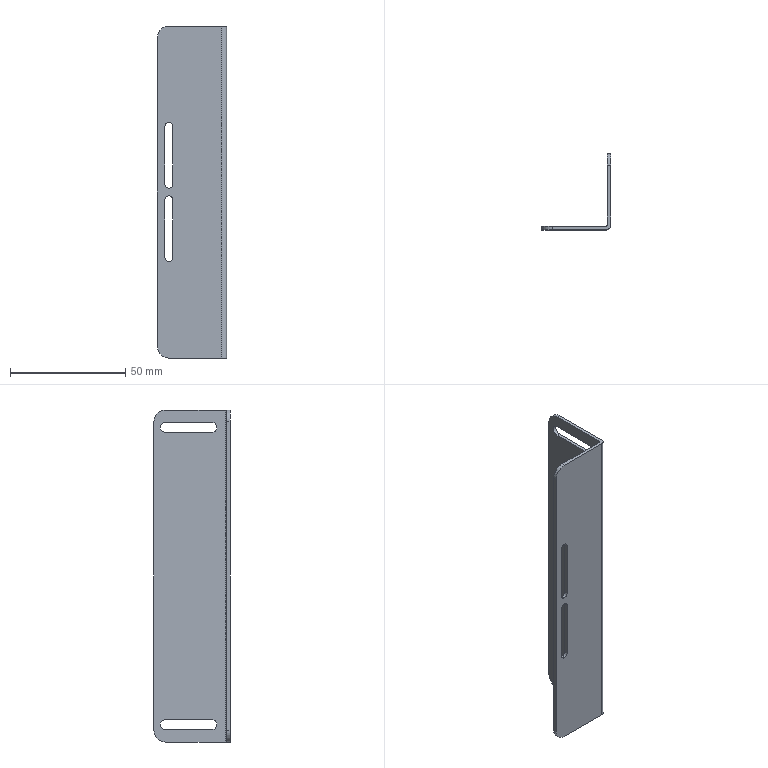Part | SolidWorks | features Fillet 3, ICE 2, Cut 1, Extrusion 1, Shell 1 | 1 solid | 32 faces | box 30 x 33 x 144 mm | volume 12527 mm3 | cylinder 16 | plane 16 | commonest cylinder face diameters 3.5 x6 4.5 x4 10 x4 1 x1 4 x1
STEP:
#1=CARTESIAN_POINT('',(6.75,1.5,43.625));
#2=VERTEX_POINT('',#1);
#3=CARTESIAN_POINT('',(5.,1.5,41.875));
#4=VERTEX_POINT('',#3);
#5=CARTESIAN_POINT('',(5.,1.5,43.625));
#6=DIRECTION('',(0.,1.,0.));
#7=DIRECTION('',(0.,0.,1.));
#8=AXIS2_PLACEMENT_3D('',#5,#6,#7);
#9=CIRCLE('',#8,1.75);
#10=EDGE_CURVE('',#2,#4,#9,.T.);
#11=ORIENTED_EDGE('',*,*,#10,.T.);
#12=CARTESIAN_POINT('',(5.,0.,41.875));
#13=VERTEX_POINT('',#12);
#14=CARTESIAN_POINT('',(5.,33.001,41.875));
#15=DIRECTION('',(0.,-1.,0.));
#16=VECTOR('',#15,1000.);
#17=LINE('',#14,#16);
#18=EDGE_CURVE('',#4,#13,#17,.T.);
#19=ORIENTED_EDGE('',*,*,#18,.T.);
#20=CARTESIAN_POINT('',(6.75,0.,43.625));
#21=VERTEX_POINT('',#20);
#22=CARTESIAN_POINT('',(5.,0.,43.625));
#23=DIRECTION('',(0.,1.,0.));
#24=DIRECTION('',(0.,0.,1.));
#25=AXIS2_PLACEMENT_3D('',#22,#23,#24);
#26=CIRCLE('',#25,1.75);
#27=EDGE_CURVE('',#21,#13,#26,.T.);
#28=ORIENTED_EDGE('',*,*,#27,.F.);
#29=CARTESIAN_POINT('',(6.75,33.001,43.625));
#30=DIRECTION('',(0.,-1.,0.));
#31=VECTOR('',#30,1000.);
#32=LINE('',#29,#31);
#33=EDGE_CURVE('',#2,#21,#32,.T.);
#34=ORIENTED_EDGE('',*,*,#33,.F.);
#35=EDGE_LOOP('',(#11,#19,#28,#34));
#36=FACE_OUTER_BOUND('',#35,.T.);
#37=CARTESIAN_POINT('',(5.,33.001,43.625));
#38=DIRECTION('',(0.,-1.,0.));
#39=DIRECTION('',(0.,0.,-1.));
#40=AXIS2_PLACEMENT_3D('',#37,#38,#39);
#41=CYLINDRICAL_SURFACE('',#40,1.75);
#42=ADVANCED_FACE('',(#36),#41,.F.);
#43=CARTESIAN_POINT('',(6.75,1.5,75.375));
#44=VERTEX_POINT('',#43);
#45=CARTESIAN_POINT('',(5.,1.5,73.625));
#46=VERTEX_POINT('',#45);
#47=CARTESIAN_POINT('',(5.,1.5,75.375));
#48=DIRECTION('',(0.,1.,0.));
#49=DIRECTION('',(0.,0.,1.));
#50=AXIS2_PLACEMENT_3D('',#47,#48,#49);
#51=CIRCLE('',#50,1.75);
#52=EDGE_CURVE('',#44,#46,#51,.T.);
#53=ORIENTED_EDGE('',*,*,#52,.T.);
#54=CARTESIAN_POINT('',(5.,0.,73.625));
#55=VERTEX_POINT('',#54);
#56=CARTESIAN_POINT('',(5.,33.001,73.625));
#57=DIRECTION('',(0.,-1.,0.));
#58=VECTOR('',#57,1000.);
#59=LINE('',#56,#58);
#60=EDGE_CURVE('',#46,#55,#59,.T.);
#61=ORIENTED_EDGE('',*,*,#60,.T.);
#62=CARTESIAN_POINT('',(6.75,0.,75.375));
#63=VERTEX_POINT('',#62);
#64=CARTESIAN_POINT('',(5.,0.,75.375));
#65=DIRECTION('',(0.,1.,0.));
#66=DIRECTION('',(0.,0.,1.));
#67=AXIS2_PLACEMENT_3D('',#64,#65,#66);
#68=CIRCLE('',#67,1.75);
#69=EDGE_CURVE('',#63,#55,#68,.T.);
#70=ORIENTED_EDGE('',*,*,#69,.F.);
#71=CARTESIAN_POINT('',(6.75,33.001,75.375));
#72=DIRECTION('',(0.,-1.,0.));
#73=VECTOR('',#72,1000.);
#74=LINE('',#71,#73);
#75=EDGE_CURVE('',#44,#63,#74,.T.);
#76=ORIENTED_EDGE('',*,*,#75,.F.);
#77=EDGE_LOOP('',(#53,#61,#70,#76));
#78=FACE_OUTER_BOUND('',#77,.T.);
#79=CARTESIAN_POINT('',(5.,33.001,75.375));
#80=DIRECTION('',(0.,-1.,0.));
#81=DIRECTION('',(0.,0.,-1.));
#82=AXIS2_PLACEMENT_3D('',#79,#80,#81);
#83=CYLINDRICAL_SURFACE('',#82,1.75);
#84=ADVANCED_FACE('',(#78),#83,.F.);
#85=ORIENTED_EDGE('',*,*,#69,.T.);
#86=CARTESIAN_POINT('',(3.25,0.,75.375));
#87=VERTEX_POINT('',#86);
#88=CARTESIAN_POINT('',(5.,0.,75.375));
#89=DIRECTION('',(0.,1.,0.));
#90=DIRECTION('',(0.,0.,1.));
#91=AXIS2_PLACEMENT_3D('',#88,#89,#90);
#92=CIRCLE('',#91,1.75);
#93=EDGE_CURVE('',#55,#87,#92,.T.);
#94=ORIENTED_EDGE('',*,*,#93,.T.);
#95=CARTESIAN_POINT('',(3.25,0.,100.375));
#96=VERTEX_POINT('',#95);
#97=CARTESIAN_POINT('',(3.25,0.,100.375));
#98=DIRECTION('',(0.,0.,1.));
#99=VECTOR('',#98,1000.);
#100=LINE('',#97,#99);
#101=EDGE_CURVE('',#87,#96,#100,.T.);
#102=ORIENTED_EDGE('',*,*,#101,.T.);
#103=CARTESIAN_POINT('',(6.75,0.,100.375));
#104=VERTEX_POINT('',#103);
#105=CARTESIAN_POINT('',(5.,0.,100.375));
#106=DIRECTION('',(0.,1.,0.));
#107=DIRECTION('',(0.,0.,1.));
#108=AXIS2_PLACEMENT_3D('',#105,#106,#107);
#109=CIRCLE('',#108,1.75);
#110=EDGE_CURVE('',#96,#104,#109,.T.);
#111=ORIENTED_EDGE('',*,*,#110,.T.);
#112=CARTESIAN_POINT('',(6.75,0.,100.375));
#113=DIRECTION('',(0.,0.,-1.));
#114=VECTOR('',#113,1000.);
#115=LINE('',#112,#114);
#116=EDGE_CURVE('',#104,#63,#115,.T.);
#117=ORIENTED_EDGE('',*,*,#116,.T.);
#118=EDGE_LOOP('',(#85,#94,#102,#111,#117));
#119=FACE_BOUND('',#118,.T.);
#120=CARTESIAN_POINT('',(5.,0.,0.));
#121=VERTEX_POINT('',#120);
#122=CARTESIAN_POINT('',(28.,0.,0.));
#123=VERTEX_POINT('',#122);
#124=CARTESIAN_POINT('',(0.,0.,0.));
#125=DIRECTION('',(1.,0.,0.));
#126=VECTOR('',#125,1000.);
#127=LINE('',#124,#126);
#128=EDGE_CURVE('',#121,#123,#127,.T.);
#129=ORIENTED_EDGE('',*,*,#128,.T.);
#130=CARTESIAN_POINT('',(28.,0.,144.));
#131=VERTEX_POINT('',#130);
#132=CARTESIAN_POINT('',(28.,0.,144.));
#133=DIRECTION('',(0.,0.,1.));
#134=VECTOR('',#133,1000.);
#135=LINE('',#132,#134);
#136=EDGE_CURVE('',#123,#131,#135,.T.);
#137=ORIENTED_EDGE('',*,*,#136,.T.);
#138=CARTESIAN_POINT('',(5.,0.,144.));
#139=VERTEX_POINT('',#138);
#140=CARTESIAN_POINT('',(0.,0.,144.));
#141=DIRECTION('',(1.,0.,0.));
#142=VECTOR('',#141,1000.);
#143=LINE('',#140,#142);
#144=EDGE_CURVE('',#139,#131,#143,.T.);
#145=ORIENTED_EDGE('',*,*,#144,.F.);
#146=CARTESIAN_POINT('',(0.,0.,139.));
#147=VERTEX_POINT('',#146);
#148=CARTESIAN_POINT('',(5.,0.,139.));
#149=DIRECTION('',(0.,-1.,0.));
#150=DIRECTION('',(0.,0.,1.));
#151=AXIS2_PLACEMENT_3D('',#148,#149,#150);
#152=CIRCLE('',#151,5.);
#153=EDGE_CURVE('',#139,#147,#152,.T.);
#154=ORIENTED_EDGE('',*,*,#153,.T.);
#155=CARTESIAN_POINT('',(0.,0.,5.));
#156=VERTEX_POINT('',#155);
#157=CARTESIAN_POINT('',(0.,0.,144.));
#158=DIRECTION('',(0.,0.,-1.));
#159=VECTOR('',#158,1000.);
#160=LINE('',#157,#159);
#161=EDGE_CURVE('',#147,#156,#160,.T.);
#162=ORIENTED_EDGE('',*,*,#161,.T.);
#163=CARTESIAN_POINT('',(5.,0.,5.));
#164=DIRECTION('',(0.,-1.,0.));
#165=DIRECTION('',(0.,0.,1.));
#166=AXIS2_PLACEMENT_3D('',#163,#164,#165);
#167=CIRCLE('',#166,5.);
#168=EDGE_CURVE('',#156,#121,#167,.T.);
#169=ORIENTED_EDGE('',*,*,#168,.T.);
#170=EDGE_LOOP('',(#129,#137,#145,#154,#162,#169));
#171=FACE_OUTER_BOUND('',#170,.T.);
#172=ORIENTED_EDGE('',*,*,#27,.T.);
#173=CARTESIAN_POINT('',(3.25,0.,43.625));
#174=VERTEX_POINT('',#173);
#175=CARTESIAN_POINT('',(5.,0.,43.625));
#176=DIRECTION('',(0.,1.,0.));
#177=DIRECTION('',(0.,0.,1.));
#178=AXIS2_PLACEMENT_3D('',#175,#176,#177);
#179=CIRCLE('',#178,1.75);
#180=EDGE_CURVE('',#13,#174,#179,.T.);
#181=ORIENTED_EDGE('',*,*,#180,.T.);
#182=CARTESIAN_POINT('',(3.25,0.,68.625));
#183=VERTEX_POINT('',#182);
#184=CARTESIAN_POINT('',(3.25,0.,68.625));
#185=DIRECTION('',(0.,0.,1.));
#186=VECTOR('',#185,1000.);
#187=LINE('',#184,#186);
#188=EDGE_CURVE('',#174,#183,#187,.T.);
#189=ORIENTED_EDGE('',*,*,#188,.T.);
#190=CARTESIAN_POINT('',(6.75,0.,68.625));
#191=VERTEX_POINT('',#190);
#192=CARTESIAN_POINT('',(5.,0.,68.625));
#193=DIRECTION('',(0.,1.,0.));
#194=DIRECTION('',(0.,0.,1.));
#195=AXIS2_PLACEMENT_3D('',#192,#193,#194);
#196=CIRCLE('',#195,1.75);
#197=EDGE_CURVE('',#183,#191,#196,.T.);
#198=ORIENTED_EDGE('',*,*,#197,.T.);
#199=CARTESIAN_POINT('',(6.75,0.,68.625));
#200=DIRECTION('',(0.,0.,-1.));
#201=VECTOR('',#200,1000.);
#202=LINE('',#199,#201);
#203=EDGE_CURVE('',#191,#21,#202,.T.);
#204=ORIENTED_EDGE('',*,*,#203,.T.);
#205=EDGE_LOOP('',(#172,#181,#189,#198,#204));
#206=FACE_BOUND('',#205,.T.);
#207=CARTESIAN_POINT('',(0.,0.,144.));
#208=DIRECTION('',(0.,1.,0.));
#209=DIRECTION('',(0.,0.,1.));
#210=AXIS2_PLACEMENT_3D('',#207,#208,#209);
#211=PLANE('',#210);
#212=ADVANCED_FACE('',(#119,#171,#206),#211,.F.);
#213=CARTESIAN_POINT('',(3.25,1.5,75.375));
#214=VERTEX_POINT('',#213);
#215=CARTESIAN_POINT('',(3.25,1.5,100.375));
#216=VERTEX_POINT('',#215);
#217=CARTESIAN_POINT('',(3.25,1.5,100.375));
#218=DIRECTION('',(0.,0.,1.));
#219=VECTOR('',#218,1000.);
#220=LINE('',#217,#219);
#221=EDGE_CURVE('',#214,#216,#220,.T.);
#222=ORIENTED_EDGE('',*,*,#221,.F.);
#223=CARTESIAN_POINT('',(5.,1.5,75.375));
#224=DIRECTION('',(0.,1.,0.));
#225=DIRECTION('',(0.,0.,1.));
#226=AXIS2_PLACEMENT_3D('',#223,#224,#225);
#227=CIRCLE('',#226,1.75);
#228=EDGE_CURVE('',#46,#214,#227,.T.);
#229=ORIENTED_EDGE('',*,*,#228,.F.);
#230=ORIENTED_EDGE('',*,*,#52,.F.);
#231=CARTESIAN_POINT('',(6.75,1.5,100.375));
#232=VERTEX_POINT('',#231);
#233=CARTESIAN_POINT('',(6.75,1.5,100.375));
#234=DIRECTION('',(0.,0.,-1.));
#235=VECTOR('',#234,1000.);
#236=LINE('',#233,#235);
#237=EDGE_CURVE('',#232,#44,#236,.T.);
#238=ORIENTED_EDGE('',*,*,#237,.F.);
#239=CARTESIAN_POINT('',(5.,1.5,100.375));
#240=DIRECTION('',(0.,1.,0.));
#241=DIRECTION('',(0.,0.,1.));
#242=AXIS2_PLACEMENT_3D('',#239,#240,#241);
#243=CIRCLE('',#242,1.75);
#244=EDGE_CURVE('',#216,#232,#243,.T.);
#245=ORIENTED_EDGE('',*,*,#244,.F.);
#246=EDGE_LOOP('',(#222,#229,#230,#238,#245));
#247=FACE_BOUND('',#246,.T.);
#248=CARTESIAN_POINT('',(5.,1.5,144.));
#249=VERTEX_POINT('',#248);
#250=CARTESIAN_POINT('',(28.,1.5,144.));
#251=VERTEX_POINT('',#250);
#252=CARTESIAN_POINT('',(0.,1.5,144.));
#253=DIRECTION('',(1.,0.,0.));
#254=VECTOR('',#253,1000.);
#255=LINE('',#252,#254);
#256=EDGE_CURVE('',#249,#251,#255,.T.);
#257=ORIENTED_EDGE('',*,*,#256,.T.);
#258=CARTESIAN_POINT('',(28.,1.5,0.));
#259=VERTEX_POINT('',#258);
#260=CARTESIAN_POINT('',(28.,1.5,0.));
#261=DIRECTION('',(0.,0.,-1.));
#262=VECTOR('',#261,1000.);
#263=LINE('',#260,#262);
#264=EDGE_CURVE('',#251,#259,#263,.T.);
#265=ORIENTED_EDGE('',*,*,#264,.T.);
#266=CARTESIAN_POINT('',(5.,1.5,0.));
#267=VERTEX_POINT('',#266);
#268=CARTESIAN_POINT('',(0.,1.5,0.));
#269=DIRECTION('',(1.,0.,0.));
#270=VECTOR('',#269,1000.);
#271=LINE('',#268,#270);
#272=EDGE_CURVE('',#267,#259,#271,.T.);
#273=ORIENTED_EDGE('',*,*,#272,.F.);
#274=CARTESIAN_POINT('',(0.,1.5,5.));
#275=VERTEX_POINT('',#274);
#276=CARTESIAN_POINT('',(5.,1.5,5.));
#277=DIRECTION('',(0.,1.,0.));
#278=DIRECTION('',(0.,0.,1.));
#279=AXIS2_PLACEMENT_3D('',#276,#277,#278);
#280=CIRCLE('',#279,5.);
#281=EDGE_CURVE('',#267,#275,#280,.T.);
#282=ORIENTED_EDGE('',*,*,#281,.T.);
#283=CARTESIAN_POINT('',(0.,1.5,139.));
#284=VERTEX_POINT('',#283);
#285=CARTESIAN_POINT('',(0.,1.5,144.));
#286=DIRECTION('',(0.,0.,-1.));
#287=VECTOR('',#286,1000.);
#288=LINE('',#285,#287);
#289=EDGE_CURVE('',#284,#275,#288,.T.);
#290=ORIENTED_EDGE('',*,*,#289,.F.);
#291=CARTESIAN_POINT('',(5.,1.5,139.));
#292=DIRECTION('',(0.,1.,0.));
#293=DIRECTION('',(0.,0.,1.));
#294=AXIS2_PLACEMENT_3D('',#291,#292,#293);
#295=CIRCLE('',#294,5.);
#296=EDGE_CURVE('',#284,#249,#295,.T.);
#297=ORIENTED_EDGE('',*,*,#296,.T.);
#298=EDGE_LOOP('',(#257,#265,#273,#282,#290,#297));
#299=FACE_OUTER_BOUND('',#298,.T.);
#300=CARTESIAN_POINT('',(3.25,1.5,43.625));
#301=VERTEX_POINT('',#300);
#302=CARTESIAN_POINT('',(3.25,1.5,68.625));
#303=VERTEX_POINT('',#302);
#304=CARTESIAN_POINT('',(3.25,1.5,68.625));
#305=DIRECTION('',(0.,0.,1.));
#306=VECTOR('',#305,1000.);
#307=LINE('',#304,#306);
#308=EDGE_CURVE('',#301,#303,#307,.T.);
#309=ORIENTED_EDGE('',*,*,#308,.F.);
#310=CARTESIAN_POINT('',(5.,1.5,43.625));
#311=DIRECTION('',(0.,1.,0.));
#312=DIRECTION('',(0.,0.,1.));
#313=AXIS2_PLACEMENT_3D('',#310,#311,#312);
#314=CIRCLE('',#313,1.75);
#315=EDGE_CURVE('',#4,#301,#314,.T.);
#316=ORIENTED_EDGE('',*,*,#315,.F.);
#317=ORIENTED_EDGE('',*,*,#10,.F.);
#318=CARTESIAN_POINT('',(6.75,1.5,68.625));
#319=VERTEX_POINT('',#318);
#320=CARTESIAN_POINT('',(6.75,1.5,68.625));
#321=DIRECTION('',(0.,0.,-1.));
#322=VECTOR('',#321,1000.);
#323=LINE('',#320,#322);
#324=EDGE_CURVE('',#319,#2,#323,.T.);
#325=ORIENTED_EDGE('',*,*,#324,.F.);
#326=CARTESIAN_POINT('',(5.,1.5,68.625));
#327=DIRECTION('',(0.,1.,0.));
#328=DIRECTION('',(0.,0.,1.));
#329=AXIS2_PLACEMENT_3D('',#326,#327,#328);
#330=CIRCLE('',#329,1.75);
#331=EDGE_CURVE('',#303,#319,#330,.T.);
#332=ORIENTED_EDGE('',*,*,#331,.F.);
#333=EDGE_LOOP('',(#309,#316,#317,#325,#332));
#334=FACE_BOUND('',#333,.T.);
#335=CARTESIAN_POINT('',(0.,1.5,144.));
#336=DIRECTION('',(0.,1.,0.));
#337=DIRECTION('',(0.,0.,1.));
#338=AXIS2_PLACEMENT_3D('',#335,#336,#337);
#339=PLANE('',#338);
#340=ADVANCED_FACE('',(#247,#299,#334),#339,.T.);
#341=CARTESIAN_POINT('',(28.5,33.,139.));
#342=VERTEX_POINT('',#341);
#343=CARTESIAN_POINT('',(28.5,33.,5.));
#344=VERTEX_POINT('',#343);
#345=CARTESIAN_POINT('',(28.5,33.,144.));
#346=DIRECTION('',(0.,0.,-1.));
#347=VECTOR('',#346,1000.);
#348=LINE('',#345,#347);
#349=EDGE_CURVE('',#342,#344,#348,.T.);
#350=ORIENTED_EDGE('',*,*,#349,.F.);
#351=CARTESIAN_POINT('',(30.,33.,139.));
#352=VERTEX_POINT('',#351);
#353=CARTESIAN_POINT('',(0.,33.,139.));
#354=DIRECTION('',(1.,0.,0.));
#355=VECTOR('',#354,1000.);
#356=LINE('',#353,#355);
#357=EDGE_CURVE('',#342,#352,#356,.T.);
#358=ORIENTED_EDGE('',*,*,#357,.T.);
#359=CARTESIAN_POINT('',(30.,33.,5.));
#360=VERTEX_POINT('',#359);
#361=CARTESIAN_POINT('',(30.,33.,144.));
#362=DIRECTION('',(0.,0.,-1.));
#363=VECTOR('',#362,1000.);
#364=LINE('',#361,#363);
#365=EDGE_CURVE('',#352,#360,#364,.T.);
#366=ORIENTED_EDGE('',*,*,#365,.T.);
#367=CARTESIAN_POINT('',(28.5,33.,5.));
#368=DIRECTION('',(-1.,0.,0.));
#369=VECTOR('',#368,1000.);
#370=LINE('',#367,#369);
#371=EDGE_CURVE('',#360,#344,#370,.T.);
#372=ORIENTED_EDGE('',*,*,#371,.T.);
#373=EDGE_LOOP('',(#350,#358,#366,#372));
#374=FACE_OUTER_BOUND('',#373,.T.);
#375=CARTESIAN_POINT('',(0.,33.,144.));
#376=DIRECTION('',(0.,-1.,0.));
#377=DIRECTION('',(0.,0.,-1.));
#378=AXIS2_PLACEMENT_3D('',#375,#376,#377);
#379=PLANE('',#378);
#380=ADVANCED_FACE('',(#374),#379,.F.);
#381=ORIENTED_EDGE('',*,*,#144,.T.);
#382=CARTESIAN_POINT('',(30.,2.,144.));
#383=VERTEX_POINT('',#382);
#384=CARTESIAN_POINT('',(28.,2.,144.));
#385=DIRECTION('',(0.,0.,1.));
#386=DIRECTION('',(-1.,0.,0.));
#387=AXIS2_PLACEMENT_3D('',#384,#385,#386);
#388=CIRCLE('',#387,2.);
#389=EDGE_CURVE('',#131,#383,#388,.T.);
#390=ORIENTED_EDGE('',*,*,#389,.T.);
#391=CARTESIAN_POINT('',(30.,28.,144.));
#392=VERTEX_POINT('',#391);
#393=CARTESIAN_POINT('',(30.,33.,144.));
#394=DIRECTION('',(0.,1.,0.));
#395=VECTOR('',#394,1000.);
#396=LINE('',#393,#395);
#397=EDGE_CURVE('',#383,#392,#396,.T.);
#398=ORIENTED_EDGE('',*,*,#397,.T.);
#399=CARTESIAN_POINT('',(28.5,28.,144.));
#400=VERTEX_POINT('',#399);
#401=CARTESIAN_POINT('',(0.,28.,144.));
#402=DIRECTION('',(-1.,0.,0.));
#403=VECTOR('',#402,1000.);
#404=LINE('',#401,#403);
#405=EDGE_CURVE('',#392,#400,#404,.T.);
#406=ORIENTED_EDGE('',*,*,#405,.T.);
#407=CARTESIAN_POINT('',(28.5,2.,144.));
#408=VERTEX_POINT('',#407);
#409=CARTESIAN_POINT('',(28.5,0.,144.));
#410=DIRECTION('',(0.,1.,0.));
#411=VECTOR('',#410,1000.);
#412=LINE('',#409,#411);
#413=EDGE_CURVE('',#408,#400,#412,.T.);
#414=ORIENTED_EDGE('',*,*,#413,.F.);
#415=CARTESIAN_POINT('',(28.,2.,144.));
#416=DIRECTION('',(0.,0.,-1.));
#417=DIRECTION('',(-1.,0.,0.));
#418=AXIS2_PLACEMENT_3D('',#415,#416,#417);
#419=CIRCLE('',#418,0.5);
#420=EDGE_CURVE('',#408,#251,#419,.T.);
#421=ORIENTED_EDGE('',*,*,#420,.T.);
#422=ORIENTED_EDGE('',*,*,#256,.F.);
#423=CARTESIAN_POINT('',(5.,0.,144.));
#424=DIRECTION('',(0.,-1.,0.));
#425=VECTOR('',#424,1000.);
#426=LINE('',#423,#425);
#427=EDGE_CURVE('',#249,#139,#426,.T.);
#428=ORIENTED_EDGE('',*,*,#427,.T.);
#429=EDGE_LOOP('',(#381,#390,#398,#406,#414,#421,#422,#428));
#430=FACE_OUTER_BOUND('',#429,.T.);
#431=CARTESIAN_POINT('',(0.,0.,144.));
#432=DIRECTION('',(0.,0.,-1.));
#433=DIRECTION('',(-1.,0.,0.));
#434=AXIS2_PLACEMENT_3D('',#431,#432,#433);
#435=PLANE('',#434);
#436=ADVANCED_FACE('',(#430),#435,.F.);
#437=CARTESIAN_POINT('',(30.,2.,0.));
#438=VERTEX_POINT('',#437);
#439=CARTESIAN_POINT('',(30.,28.,0.));
#440=VERTEX_POINT('',#439);
#441=CARTESIAN_POINT('',(30.,33.,0.));
#442=DIRECTION('',(0.,1.,0.));
#443=VECTOR('',#442,1000.);
#444=LINE('',#441,#443);
#445=EDGE_CURVE('',#438,#440,#444,.T.);
#446=ORIENTED_EDGE('',*,*,#445,.F.);
#447=CARTESIAN_POINT('',(28.,2.,0.));
#448=DIRECTION('',(0.,0.,-1.));
#449=DIRECTION('',(-1.,0.,0.));
#450=AXIS2_PLACEMENT_3D('',#447,#448,#449);
#451=CIRCLE('',#450,2.);
#452=EDGE_CURVE('',#438,#123,#451,.T.);
#453=ORIENTED_EDGE('',*,*,#452,.T.);
#454=ORIENTED_EDGE('',*,*,#128,.F.);
#455=CARTESIAN_POINT('',(5.,1.5,0.));
#456=DIRECTION('',(0.,1.,0.));
#457=VECTOR('',#456,1000.);
#458=LINE('',#455,#457);
#459=EDGE_CURVE('',#121,#267,#458,.T.);
#460=ORIENTED_EDGE('',*,*,#459,.T.);
#461=ORIENTED_EDGE('',*,*,#272,.T.);
#462=CARTESIAN_POINT('',(28.5,2.,0.));
#463=VERTEX_POINT('',#462);
#464=CARTESIAN_POINT('',(28.,2.,0.));
#465=DIRECTION('',(0.,0.,1.));
#466=DIRECTION('',(-1.,0.,0.));
#467=AXIS2_PLACEMENT_3D('',#464,#465,#466);
#468=CIRCLE('',#467,0.5);
#469=EDGE_CURVE('',#259,#463,#468,.T.);
#470=ORIENTED_EDGE('',*,*,#469,.T.);
#471=CARTESIAN_POINT('',(28.5,28.,0.));
#472=VERTEX_POINT('',#471);
#473=CARTESIAN_POINT('',(28.5,0.,0.));
#474=DIRECTION('',(0.,1.,0.));
#475=VECTOR('',#474,1000.);
#476=LINE('',#473,#475);
#477=EDGE_CURVE('',#463,#472,#476,.T.);
#478=ORIENTED_EDGE('',*,*,#477,.T.);
#479=CARTESIAN_POINT('',(30.,28.,0.));
#480=DIRECTION('',(1.,0.,0.));
#481=VECTOR('',#480,1000.);
#482=LINE('',#479,#481);
#483=EDGE_CURVE('',#472,#440,#482,.T.);
#484=ORIENTED_EDGE('',*,*,#483,.T.);
#485=EDGE_LOOP('',(#446,#453,#454,#460,#461,#470,#478,#484));
#486=FACE_OUTER_BOUND('',#485,.T.);
#487=CARTESIAN_POINT('',(0.,0.,0.));
#488=DIRECTION('',(0.,0.,-1.));
#489=DIRECTION('',(-1.,0.,0.));
#490=AXIS2_PLACEMENT_3D('',#487,#488,#489);
#491=PLANE('',#490);
#492=ADVANCED_FACE('',(#486),#491,.T.);
#493=ORIENTED_EDGE('',*,*,#289,.T.);
#494=CARTESIAN_POINT('',(0.,0.,5.));
#495=DIRECTION('',(0.,-1.,0.));
#496=VECTOR('',#495,1000.);
#497=LINE('',#494,#496);
#498=EDGE_CURVE('',#275,#156,#497,.T.);
#499=ORIENTED_EDGE('',*,*,#498,.T.);
#500=ORIENTED_EDGE('',*,*,#161,.F.);
#501=CARTESIAN_POINT('',(0.,0.,139.));
#502=DIRECTION('',(0.,1.,0.));
#503=VECTOR('',#502,1000.);
#504=LINE('',#501,#503);
#505=EDGE_CURVE('',#147,#284,#504,.T.);
#506=ORIENTED_EDGE('',*,*,#505,.T.);
#507=EDGE_LOOP('',(#493,#499,#500,#506));
#508=FACE_OUTER_BOUND('',#507,.T.);
#509=CARTESIAN_POINT('',(0.,0.,144.));
#510=DIRECTION('',(1.,0.,0.));
#511=DIRECTION('',(0.,0.,-1.));
#512=AXIS2_PLACEMENT_3D('',#509,#510,#511);
#513=PLANE('',#512);
#514=ADVANCED_FACE('',(#508),#513,.F.);
#515=CARTESIAN_POINT('',(30.,8.,138.75));
#516=VERTEX_POINT('',#515);
#517=CARTESIAN_POINT('',(30.,28.,138.75));
#518=VERTEX_POINT('',#517);
#519=CARTESIAN_POINT('',(30.,28.,138.75));
#520=DIRECTION('',(0.,1.,0.));
#521=VECTOR('',#520,1000.);
#522=LINE('',#519,#521);
#523=EDGE_CURVE('',#516,#518,#522,.T.);
#524=ORIENTED_EDGE('',*,*,#523,.T.);
#525=CARTESIAN_POINT('',(30.,28.,134.25));
#526=VERTEX_POINT('',#525);
#527=CARTESIAN_POINT('',(30.,28.,136.5));
#528=DIRECTION('',(-1.,0.,0.));
#529=DIRECTION('',(0.,0.,1.));
#530=AXIS2_PLACEMENT_3D('',#527,#528,#529);
#531=CIRCLE('',#530,2.25);
#532=EDGE_CURVE('',#518,#526,#531,.T.);
#533=ORIENTED_EDGE('',*,*,#532,.T.);
#534=CARTESIAN_POINT('',(30.,8.,134.25));
#535=VERTEX_POINT('',#534);
#536=CARTESIAN_POINT('',(30.,28.,134.25));
#537=DIRECTION('',(0.,-1.,0.));
#538=VECTOR('',#537,1000.);
#539=LINE('',#536,#538);
#540=EDGE_CURVE('',#526,#535,#539,.T.);
#541=ORIENTED_EDGE('',*,*,#540,.T.);
#542=CARTESIAN_POINT('',(30.,8.,136.5));
#543=DIRECTION('',(-1.,0.,0.));
#544=DIRECTION('',(0.,0.,1.));
#545=AXIS2_PLACEMENT_3D('',#542,#543,#544);
#546=CIRCLE('',#545,2.25);
#547=EDGE_CURVE('',#535,#516,#546,.T.);
#548=ORIENTED_EDGE('',*,*,#547,.T.);
#549=EDGE_LOOP('',(#524,#533,#541,#548));
#550=FACE_BOUND('',#549,.T.);
#551=CARTESIAN_POINT('',(30.,28.,5.25));
#552=VERTEX_POINT('',#551);
#553=CARTESIAN_POINT('',(30.,8.,5.25));
#554=VERTEX_POINT('',#553);
#555=CARTESIAN_POINT('',(30.,8.,5.25));
#556=DIRECTION('',(0.,-1.,0.));
#557=VECTOR('',#556,1000.);
#558=LINE('',#555,#557);
#559=EDGE_CURVE('',#552,#554,#558,.T.);
#560=ORIENTED_EDGE('',*,*,#559,.T.);
#561=CARTESIAN_POINT('',(30.,8.,9.75));
#562=VERTEX_POINT('',#561);
#563=CARTESIAN_POINT('',(30.,8.,7.5));
#564=DIRECTION('',(-1.,0.,0.));
#565=DIRECTION('',(0.,0.,1.));
#566=AXIS2_PLACEMENT_3D('',#563,#564,#565);
#567=CIRCLE('',#566,2.25);
#568=EDGE_CURVE('',#554,#562,#567,.T.);
#569=ORIENTED_EDGE('',*,*,#568,.T.);
#570=CARTESIAN_POINT('',(30.,28.,9.75));
#571=VERTEX_POINT('',#570);
#572=CARTESIAN_POINT('',(30.,8.,9.75));
#573=DIRECTION('',(0.,1.,0.));
#574=VECTOR('',#573,1000.);
#575=LINE('',#572,#574);
#576=EDGE_CURVE('',#562,#571,#575,.T.);
#577=ORIENTED_EDGE('',*,*,#576,.T.);
#578=CARTESIAN_POINT('',(30.,28.,7.5));
#579=DIRECTION('',(-1.,0.,0.));
#580=DIRECTION('',(0.,0.,1.));
#581=AXIS2_PLACEMENT_3D('',#578,#579,#580);
#582=CIRCLE('',#581,2.25);
#583=EDGE_CURVE('',#571,#552,#582,.T.);
#584=ORIENTED_EDGE('',*,*,#583,.T.);
#585=EDGE_LOOP('',(#560,#569,#577,#584));
#586=FACE_BOUND('',#585,.T.);
#587=ORIENTED_EDGE('',*,*,#397,.F.);
#588=CARTESIAN_POINT('',(30.,2.,144.));
#589=DIRECTION('',(0.,0.,-1.));
#590=VECTOR('',#589,1000.);
#591=LINE('',#588,#590);
#592=EDGE_CURVE('',#383,#438,#591,.T.);
#593=ORIENTED_EDGE('',*,*,#592,.T.);
#594=ORIENTED_EDGE('',*,*,#445,.T.);
#595=CARTESIAN_POINT('',(30.,28.,5.));
#596=DIRECTION('',(1.,0.,0.));
#597=DIRECTION('',(0.,-1.,0.));
#598=AXIS2_PLACEMENT_3D('',#595,#596,#597);
#599=CIRCLE('',#598,5.);
#600=EDGE_CURVE('',#440,#360,#599,.T.);
#601=ORIENTED_EDGE('',*,*,#600,.T.);
#602=ORIENTED_EDGE('',*,*,#365,.F.);
#603=CARTESIAN_POINT('',(30.,28.,139.));
#604=DIRECTION('',(1.,0.,0.));
#605=DIRECTION('',(0.,-1.,0.));
#606=AXIS2_PLACEMENT_3D('',#603,#604,#605);
#607=CIRCLE('',#606,5.);
#608=EDGE_CURVE('',#352,#392,#607,.T.);
#609=ORIENTED_EDGE('',*,*,#608,.T.);
#610=EDGE_LOOP('',(#587,#593,#594,#601,#602,#609));
#611=FACE_OUTER_BOUND('',#610,.T.);
#612=CARTESIAN_POINT('',(30.,33.,144.));
#613=DIRECTION('',(-1.,0.,0.));
#614=DIRECTION('',(0.,-1.,0.));
#615=AXIS2_PLACEMENT_3D('',#612,#613,#614);
#616=PLANE('',#615);
#617=ADVANCED_FACE('',(#550,#586,#611),#616,.F.);
#618=CARTESIAN_POINT('',(28.5,28.,138.75));
#619=VERTEX_POINT('',#618);
#620=CARTESIAN_POINT('',(28.5,28.,134.25));
#621=VERTEX_POINT('',#620);
#622=CARTESIAN_POINT('',(28.5,28.,136.5));
#623=DIRECTION('',(-1.,0.,0.));
#624=DIRECTION('',(0.,0.,1.));
#625=AXIS2_PLACEMENT_3D('',#622,#623,#624);
#626=CIRCLE('',#625,2.25);
#627=EDGE_CURVE('',#619,#621,#626,.T.);
#628=ORIENTED_EDGE('',*,*,#627,.F.);
#629=CARTESIAN_POINT('',(28.5,8.,138.75));
#630=VERTEX_POINT('',#629);
#631=CARTESIAN_POINT('',(28.5,28.,138.75));
#632=DIRECTION('',(0.,1.,0.));
#633=VECTOR('',#632,1000.);
#634=LINE('',#631,#633);
#635=EDGE_CURVE('',#630,#619,#634,.T.);
#636=ORIENTED_EDGE('',*,*,#635,.F.);
#637=CARTESIAN_POINT('',(28.5,8.,134.25));
#638=VERTEX_POINT('',#637);
#639=CARTESIAN_POINT('',(28.5,8.,136.5));
#640=DIRECTION('',(-1.,0.,0.));
#641=DIRECTION('',(0.,0.,1.));
#642=AXIS2_PLACEMENT_3D('',#639,#640,#641);
#643=CIRCLE('',#642,2.25);
#644=EDGE_CURVE('',#638,#630,#643,.T.);
#645=ORIENTED_EDGE('',*,*,#644,.F.);
#646=CARTESIAN_POINT('',(28.5,28.,134.25));
#647=DIRECTION('',(0.,-1.,0.));
#648=VECTOR('',#647,1000.);
#649=LINE('',#646,#648);
#650=EDGE_CURVE('',#621,#638,#649,.T.);
#651=ORIENTED_EDGE('',*,*,#650,.F.);
#652=EDGE_LOOP('',(#628,#636,#645,#651));
#653=FACE_BOUND('',#652,.T.);
#654=CARTESIAN_POINT('',(28.5,8.,5.25));
#655=VERTEX_POINT('',#654);
#656=CARTESIAN_POINT('',(28.5,8.,9.75));
#657=VERTEX_POINT('',#656);
#658=CARTESIAN_POINT('',(28.5,8.,7.5));
#659=DIRECTION('',(-1.,0.,0.));
#660=DIRECTION('',(0.,0.,1.));
#661=AXIS2_PLACEMENT_3D('',#658,#659,#660);
#662=CIRCLE('',#661,2.25);
#663=EDGE_CURVE('',#655,#657,#662,.T.);
#664=ORIENTED_EDGE('',*,*,#663,.F.);
#665=CARTESIAN_POINT('',(28.5,28.,5.25));
#666=VERTEX_POINT('',#665);
#667=CARTESIAN_POINT('',(28.5,8.,5.25));
#668=DIRECTION('',(0.,-1.,0.));
#669=VECTOR('',#668,1000.);
#670=LINE('',#667,#669);
#671=EDGE_CURVE('',#666,#655,#670,.T.);
#672=ORIENTED_EDGE('',*,*,#671,.F.);
#673=CARTESIAN_POINT('',(28.5,28.,9.75));
#674=VERTEX_POINT('',#673);
#675=CARTESIAN_POINT('',(28.5,28.,7.5));
#676=DIRECTION('',(-1.,0.,0.));
#677=DIRECTION('',(0.,0.,1.));
#678=AXIS2_PLACEMENT_3D('',#675,#676,#677);
#679=CIRCLE('',#678,2.25);
#680=EDGE_CURVE('',#674,#666,#679,.T.);
#681=ORIENTED_EDGE('',*,*,#680,.F.);
#682=CARTESIAN_POINT('',(28.5,8.,9.75));
#683=DIRECTION('',(0.,1.,0.));
#684=VECTOR('',#683,1000.);
#685=LINE('',#682,#684);
#686=EDGE_CURVE('',#657,#674,#685,.T.);
#687=ORIENTED_EDGE('',*,*,#686,.F.);
#688=EDGE_LOOP('',(#664,#672,#681,#687));
#689=FACE_BOUND('',#688,.T.);
#690=ORIENTED_EDGE('',*,*,#477,.F.);
#691=CARTESIAN_POINT('',(28.5,2.,144.));
#692=DIRECTION('',(0.,0.,1.));
#693=VECTOR('',#692,1000.);
#694=LINE('',#691,#693);
#695=EDGE_CURVE('',#463,#408,#694,.T.);
#696=ORIENTED_EDGE('',*,*,#695,.T.);
#697=ORIENTED_EDGE('',*,*,#413,.T.);
#698=CARTESIAN_POINT('',(28.5,28.,139.));
#699=DIRECTION('',(-1.,0.,0.));
#700=DIRECTION('',(0.,-1.,0.));
#701=AXIS2_PLACEMENT_3D('',#698,#699,#700);
#702=CIRCLE('',#701,5.);
#703=EDGE_CURVE('',#400,#342,#702,.T.);
#704=ORIENTED_EDGE('',*,*,#703,.T.);
#705=ORIENTED_EDGE('',*,*,#349,.T.);
#706=CARTESIAN_POINT('',(28.5,28.,5.));
#707=DIRECTION('',(-1.,0.,0.));
#708=DIRECTION('',(0.,-1.,0.));
#709=AXIS2_PLACEMENT_3D('',#706,#707,#708);
#710=CIRCLE('',#709,5.);
#711=EDGE_CURVE('',#344,#472,#710,.T.);
#712=ORIENTED_EDGE('',*,*,#711,.T.);
#713=EDGE_LOOP('',(#690,#696,#697,#704,#705,#712));
#714=FACE_OUTER_BOUND('',#713,.T.);
#715=CARTESIAN_POINT('',(28.5,33.,144.));
#716=DIRECTION('',(-1.,0.,0.));
#717=DIRECTION('',(0.,-1.,0.));
#718=AXIS2_PLACEMENT_3D('',#715,#716,#717);
#719=PLANE('',#718);
#720=ADVANCED_FACE('',(#653,#689,#714),#719,.T.);
#721=ORIENTED_EDGE('',*,*,#608,.F.);
#722=ORIENTED_EDGE('',*,*,#357,.F.);
#723=ORIENTED_EDGE('',*,*,#703,.F.);
#724=ORIENTED_EDGE('',*,*,#405,.F.);
#725=EDGE_LOOP('',(#721,#722,#723,#724));
#726=FACE_OUTER_BOUND('',#725,.T.);
#727=CARTESIAN_POINT('',(0.,28.,139.));
#728=DIRECTION('',(-1.,0.,0.));
#729=DIRECTION('',(0.,0.,1.));
#730=AXIS2_PLACEMENT_3D('',#727,#728,#729);
#731=CYLINDRICAL_SURFACE('',#730,5.);
#732=ADVANCED_FACE('',(#726),#731,.T.);
#733=ORIENTED_EDGE('',*,*,#600,.F.);
#734=ORIENTED_EDGE('',*,*,#483,.F.);
#735=ORIENTED_EDGE('',*,*,#711,.F.);
#736=ORIENTED_EDGE('',*,*,#371,.F.);
#737=EDGE_LOOP('',(#733,#734,#735,#736));
#738=FACE_OUTER_BOUND('',#737,.T.);
#739=CARTESIAN_POINT('',(0.,28.,5.));
#740=DIRECTION('',(1.,0.,0.));
#741=DIRECTION('',(0.,0.,-1.));
#742=AXIS2_PLACEMENT_3D('',#739,#740,#741);
#743=CYLINDRICAL_SURFACE('',#742,5.);
#744=ADVANCED_FACE('',(#738),#743,.T.);
#745=ORIENTED_EDGE('',*,*,#281,.F.);
#746=ORIENTED_EDGE('',*,*,#459,.F.);
#747=ORIENTED_EDGE('',*,*,#168,.F.);
#748=ORIENTED_EDGE('',*,*,#498,.F.);
#749=EDGE_LOOP('',(#745,#746,#747,#748));
#750=FACE_OUTER_BOUND('',#749,.T.);
#751=CARTESIAN_POINT('',(5.,0.,5.));
#752=DIRECTION('',(0.,1.,0.));
#753=DIRECTION('',(0.,0.,1.));
#754=AXIS2_PLACEMENT_3D('',#751,#752,#753);
#755=CYLINDRICAL_SURFACE('',#754,5.);
#756=ADVANCED_FACE('',(#750),#755,.T.);
#757=ORIENTED_EDGE('',*,*,#296,.F.);
#758=ORIENTED_EDGE('',*,*,#505,.F.);
#759=ORIENTED_EDGE('',*,*,#153,.F.);
#760=ORIENTED_EDGE('',*,*,#427,.F.);
#761=EDGE_LOOP('',(#757,#758,#759,#760));
#762=FACE_OUTER_BOUND('',#761,.T.);
#763=CARTESIAN_POINT('',(5.,0.,139.));
#764=DIRECTION('',(0.,-1.,0.));
#765=DIRECTION('',(0.,0.,-1.));
#766=AXIS2_PLACEMENT_3D('',#763,#764,#765);
#767=CYLINDRICAL_SURFACE('',#766,5.);
#768=ADVANCED_FACE('',(#762),#767,.T.);
#769=ORIENTED_EDGE('',*,*,#420,.F.);
#770=ORIENTED_EDGE('',*,*,#695,.F.);
#771=ORIENTED_EDGE('',*,*,#469,.F.);
#772=ORIENTED_EDGE('',*,*,#264,.F.);
#773=EDGE_LOOP('',(#769,#770,#771,#772));
#774=FACE_OUTER_BOUND('',#773,.T.);
#775=CARTESIAN_POINT('',(28.,2.,144.));
#776=DIRECTION('',(0.,0.,1.));
#777=DIRECTION('',(1.,0.,0.));
#778=AXIS2_PLACEMENT_3D('',#775,#776,#777);
#779=CYLINDRICAL_SURFACE('',#778,0.5);
#780=ADVANCED_FACE('',(#774),#779,.F.);
#781=ORIENTED_EDGE('',*,*,#389,.F.);
#782=ORIENTED_EDGE('',*,*,#136,.F.);
#783=ORIENTED_EDGE('',*,*,#452,.F.);
#784=ORIENTED_EDGE('',*,*,#592,.F.);
#785=EDGE_LOOP('',(#781,#782,#783,#784));
#786=FACE_OUTER_BOUND('',#785,.T.);
#787=CARTESIAN_POINT('',(28.,2.,144.));
#788=DIRECTION('',(0.,0.,-1.));
#789=DIRECTION('',(-1.,0.,0.));
#790=AXIS2_PLACEMENT_3D('',#787,#788,#789);
#791=CYLINDRICAL_SURFACE('',#790,2.);
#792=ADVANCED_FACE('',(#786),#791,.T.);
#793=ORIENTED_EDGE('',*,*,#663,.T.);
#794=CARTESIAN_POINT('',(30.,8.,9.75));
#795=DIRECTION('',(-1.,0.,0.));
#796=VECTOR('',#795,1000.);
#797=LINE('',#794,#796);
#798=EDGE_CURVE('',#562,#657,#797,.T.);
#799=ORIENTED_EDGE('',*,*,#798,.F.);
#800=ORIENTED_EDGE('',*,*,#568,.F.);
#801=CARTESIAN_POINT('',(30.,8.,5.25));
#802=DIRECTION('',(-1.,0.,0.));
#803=VECTOR('',#802,1000.);
#804=LINE('',#801,#803);
#805=EDGE_CURVE('',#554,#655,#804,.T.);
#806=ORIENTED_EDGE('',*,*,#805,.T.);
#807=EDGE_LOOP('',(#793,#799,#800,#806));
#808=FACE_OUTER_BOUND('',#807,.T.);
#809=CARTESIAN_POINT('',(30.,8.,7.5));
#810=DIRECTION('',(-1.,0.,0.));
#811=DIRECTION('',(0.,0.,1.));
#812=AXIS2_PLACEMENT_3D('',#809,#810,#811);
#813=CYLINDRICAL_SURFACE('',#812,2.25);
#814=ADVANCED_FACE('',(#808),#813,.F.);
#815=ORIENTED_EDGE('',*,*,#671,.T.);
#816=ORIENTED_EDGE('',*,*,#805,.F.);
#817=ORIENTED_EDGE('',*,*,#559,.F.);
#818=CARTESIAN_POINT('',(30.,28.,5.25));
#819=DIRECTION('',(-1.,0.,0.));
#820=VECTOR('',#819,1000.);
#821=LINE('',#818,#820);
#822=EDGE_CURVE('',#552,#666,#821,.T.);
#823=ORIENTED_EDGE('',*,*,#822,.T.);
#824=EDGE_LOOP('',(#815,#816,#817,#823));
#825=FACE_OUTER_BOUND('',#824,.T.);
#826=CARTESIAN_POINT('',(30.,8.,5.25));
#827=DIRECTION('',(0.,0.,-1.));
#828=DIRECTION('',(-1.,0.,0.));
#829=AXIS2_PLACEMENT_3D('',#826,#827,#828);
#830=PLANE('',#829);
#831=ADVANCED_FACE('',(#825),#830,.F.);
#832=ORIENTED_EDGE('',*,*,#680,.T.);
#833=ORIENTED_EDGE('',*,*,#822,.F.);
#834=ORIENTED_EDGE('',*,*,#583,.F.);
#835=CARTESIAN_POINT('',(30.,28.,9.75));
#836=DIRECTION('',(-1.,0.,0.));
#837=VECTOR('',#836,1000.);
#838=LINE('',#835,#837);
#839=EDGE_CURVE('',#571,#674,#838,.T.);
#840=ORIENTED_EDGE('',*,*,#839,.T.);
#841=EDGE_LOOP('',(#832,#833,#834,#840));
#842=FACE_OUTER_BOUND('',#841,.T.);
#843=CARTESIAN_POINT('',(30.,28.,7.5));
#844=DIRECTION('',(-1.,0.,0.));
#845=DIRECTION('',(0.,0.,1.));
#846=AXIS2_PLACEMENT_3D('',#843,#844,#845);
#847=CYLINDRICAL_SURFACE('',#846,2.25);
#848=ADVANCED_FACE('',(#842),#847,.F.);
#849=ORIENTED_EDGE('',*,*,#686,.T.);
#850=ORIENTED_EDGE('',*,*,#839,.F.);
#851=ORIENTED_EDGE('',*,*,#576,.F.);
#852=ORIENTED_EDGE('',*,*,#798,.T.);
#853=EDGE_LOOP('',(#849,#850,#851,#852));
#854=FACE_OUTER_BOUND('',#853,.T.);
#855=CARTESIAN_POINT('',(30.,8.,9.75));
#856=DIRECTION('',(0.,0.,1.));
#857=DIRECTION('',(1.,0.,0.));
#858=AXIS2_PLACEMENT_3D('',#855,#856,#857);
#859=PLANE('',#858);
#860=ADVANCED_FACE('',(#854),#859,.F.);
#861=ORIENTED_EDGE('',*,*,#627,.T.);
#862=CARTESIAN_POINT('',(30.,28.,134.25));
#863=DIRECTION('',(-1.,0.,0.));
#864=VECTOR('',#863,1000.);
#865=LINE('',#862,#864);
#866=EDGE_CURVE('',#526,#621,#865,.T.);
#867=ORIENTED_EDGE('',*,*,#866,.F.);
#868=ORIENTED_EDGE('',*,*,#532,.F.);
#869=CARTESIAN_POINT('',(30.,28.,138.75));
#870=DIRECTION('',(-1.,0.,0.));
#871=VECTOR('',#870,1000.);
#872=LINE('',#869,#871);
#873=EDGE_CURVE('',#518,#619,#872,.T.);
#874=ORIENTED_EDGE('',*,*,#873,.T.);
#875=EDGE_LOOP('',(#861,#867,#868,#874));
#876=FACE_OUTER_BOUND('',#875,.T.);
#877=CARTESIAN_POINT('',(30.,28.,136.5));
#878=DIRECTION('',(-1.,0.,0.));
#879=DIRECTION('',(0.,0.,1.));
#880=AXIS2_PLACEMENT_3D('',#877,#878,#879);
#881=CYLINDRICAL_SURFACE('',#880,2.25);
#882=ADVANCED_FACE('',(#876),#881,.F.);
#883=ORIENTED_EDGE('',*,*,#635,.T.);
#884=ORIENTED_EDGE('',*,*,#873,.F.);
#885=ORIENTED_EDGE('',*,*,#523,.F.);
#886=CARTESIAN_POINT('',(30.,8.,138.75));
#887=DIRECTION('',(-1.,0.,0.));
#888=VECTOR('',#887,1000.);
#889=LINE('',#886,#888);
#890=EDGE_CURVE('',#516,#630,#889,.T.);
#891=ORIENTED_EDGE('',*,*,#890,.T.);
#892=EDGE_LOOP('',(#883,#884,#885,#891));
#893=FACE_OUTER_BOUND('',#892,.T.);
#894=CARTESIAN_POINT('',(30.,28.,138.75));
#895=DIRECTION('',(0.,0.,1.));
#896=DIRECTION('',(1.,0.,0.));
#897=AXIS2_PLACEMENT_3D('',#894,#895,#896);
#898=PLANE('',#897);
#899=ADVANCED_FACE('',(#893),#898,.F.);
#900=ORIENTED_EDGE('',*,*,#644,.T.);
#901=ORIENTED_EDGE('',*,*,#890,.F.);
#902=ORIENTED_EDGE('',*,*,#547,.F.);
#903=CARTESIAN_POINT('',(30.,8.,134.25));
#904=DIRECTION('',(-1.,0.,0.));
#905=VECTOR('',#904,1000.);
#906=LINE('',#903,#905);
#907=EDGE_CURVE('',#535,#638,#906,.T.);
#908=ORIENTED_EDGE('',*,*,#907,.T.);
#909=EDGE_LOOP('',(#900,#901,#902,#908));
#910=FACE_OUTER_BOUND('',#909,.T.);
#911=CARTESIAN_POINT('',(30.,8.,136.5));
#912=DIRECTION('',(-1.,0.,0.));
#913=DIRECTION('',(0.,0.,1.));
#914=AXIS2_PLACEMENT_3D('',#911,#912,#913);
#915=CYLINDRICAL_SURFACE('',#914,2.25);
#916=ADVANCED_FACE('',(#910),#915,.F.);
#917=ORIENTED_EDGE('',*,*,#650,.T.);
#918=ORIENTED_EDGE('',*,*,#907,.F.);
#919=ORIENTED_EDGE('',*,*,#540,.F.);
#920=ORIENTED_EDGE('',*,*,#866,.T.);
#921=EDGE_LOOP('',(#917,#918,#919,#920));
#922=FACE_OUTER_BOUND('',#921,.T.);
#923=CARTESIAN_POINT('',(30.,28.,134.25));
#924=DIRECTION('',(0.,0.,-1.));
#925=DIRECTION('',(-1.,0.,0.));
#926=AXIS2_PLACEMENT_3D('',#923,#924,#925);
#927=PLANE('',#926);
#928=ADVANCED_FACE('',(#922),#927,.F.);
#929=ORIENTED_EDGE('',*,*,#221,.T.);
#930=CARTESIAN_POINT('',(3.25,33.001,100.375));
#931=DIRECTION('',(0.,-1.,0.));
#932=VECTOR('',#931,1000.);
#933=LINE('',#930,#932);
#934=EDGE_CURVE('',#216,#96,#933,.T.);
#935=ORIENTED_EDGE('',*,*,#934,.T.);
#936=ORIENTED_EDGE('',*,*,#101,.F.);
#937=CARTESIAN_POINT('',(3.25,33.001,75.375));
#938=DIRECTION('',(0.,-1.,0.));
#939=VECTOR('',#938,1000.);
#940=LINE('',#937,#939);
#941=EDGE_CURVE('',#214,#87,#940,.T.);
#942=ORIENTED_EDGE('',*,*,#941,.F.);
#943=EDGE_LOOP('',(#929,#935,#936,#942));
#944=FACE_OUTER_BOUND('',#943,.T.);
#945=CARTESIAN_POINT('',(3.25,33.001,100.375));
#946=DIRECTION('',(1.,0.,0.));
#947=DIRECTION('',(0.,0.,-1.));
#948=AXIS2_PLACEMENT_3D('',#945,#946,#947);
#949=PLANE('',#948);
#950=ADVANCED_FACE('',(#944),#949,.T.);
#951=ORIENTED_EDGE('',*,*,#237,.T.);
#952=ORIENTED_EDGE('',*,*,#75,.T.);
#953=ORIENTED_EDGE('',*,*,#116,.F.);
#954=CARTESIAN_POINT('',(6.75,33.001,100.375));
#955=DIRECTION('',(0.,-1.,0.));
#956=VECTOR('',#955,1000.);
#957=LINE('',#954,#956);
#958=EDGE_CURVE('',#232,#104,#957,.T.);
#959=ORIENTED_EDGE('',*,*,#958,.F.);
#960=EDGE_LOOP('',(#951,#952,#953,#959));
#961=FACE_OUTER_BOUND('',#960,.T.);
#962=CARTESIAN_POINT('',(6.75,33.001,100.375));
#963=DIRECTION('',(-1.,0.,0.));
#964=DIRECTION('',(0.,0.,1.));
#965=AXIS2_PLACEMENT_3D('',#962,#963,#964);
#966=PLANE('',#965);
#967=ADVANCED_FACE('',(#961),#966,.T.);
#968=ORIENTED_EDGE('',*,*,#244,.T.);
#969=ORIENTED_EDGE('',*,*,#958,.T.);
#970=ORIENTED_EDGE('',*,*,#110,.F.);
#971=ORIENTED_EDGE('',*,*,#934,.F.);
#972=EDGE_LOOP('',(#968,#969,#970,#971));
#973=FACE_OUTER_BOUND('',#972,.T.);
#974=CARTESIAN_POINT('',(5.,33.001,100.375));
#975=DIRECTION('',(0.,-1.,0.));
#976=DIRECTION('',(0.,0.,-1.));
#977=AXIS2_PLACEMENT_3D('',#974,#975,#976);
#978=CYLINDRICAL_SURFACE('',#977,1.75);
#979=ADVANCED_FACE('',(#973),#978,.F.);
#980=ORIENTED_EDGE('',*,*,#308,.T.);
#981=CARTESIAN_POINT('',(3.25,33.001,68.625));
#982=DIRECTION('',(0.,-1.,0.));
#983=VECTOR('',#982,1000.);
#984=LINE('',#981,#983);
#985=EDGE_CURVE('',#303,#183,#984,.T.);
#986=ORIENTED_EDGE('',*,*,#985,.T.);
#987=ORIENTED_EDGE('',*,*,#188,.F.);
#988=CARTESIAN_POINT('',(3.25,33.001,43.625));
#989=DIRECTION('',(0.,-1.,0.));
#990=VECTOR('',#989,1000.);
#991=LINE('',#988,#990);
#992=EDGE_CURVE('',#301,#174,#991,.T.);
#993=ORIENTED_EDGE('',*,*,#992,.F.);
#994=EDGE_LOOP('',(#980,#986,#987,#993));
#995=FACE_OUTER_BOUND('',#994,.T.);
#996=CARTESIAN_POINT('',(3.25,33.001,68.625));
#997=DIRECTION('',(1.,0.,0.));
#998=DIRECTION('',(0.,0.,-1.));
#999=AXIS2_PLACEMENT_3D('',#996,#997,#998);
#1000=PLANE('',#999);
#1001=ADVANCED_FACE('',(#995),#1000,.T.);
#1002=ORIENTED_EDGE('',*,*,#324,.T.);
#1003=ORIENTED_EDGE('',*,*,#33,.T.);
#1004=ORIENTED_EDGE('',*,*,#203,.F.);
#1005=CARTESIAN_POINT('',(6.75,33.001,68.625));
#1006=DIRECTION('',(0.,-1.,0.));
#1007=VECTOR('',#1006,1000.);
#1008=LINE('',#1005,#1007);
#1009=EDGE_CURVE('',#319,#191,#1008,.T.);
#1010=ORIENTED_EDGE('',*,*,#1009,.F.);
#1011=EDGE_LOOP('',(#1002,#1003,#1004,#1010));
#1012=FACE_OUTER_BOUND('',#1011,.T.);
#1013=CARTESIAN_POINT('',(6.75,33.001,68.625));
#1014=DIRECTION('',(-1.,0.,0.));
#1015=DIRECTION('',(0.,0.,1.));
#1016=AXIS2_PLACEMENT_3D('',#1013,#1014,#1015);
#1017=PLANE('',#1016);
#1018=ADVANCED_FACE('',(#1012),#1017,.T.);
#1019=ORIENTED_EDGE('',*,*,#331,.T.);
#1020=ORIENTED_EDGE('',*,*,#1009,.T.);
#1021=ORIENTED_EDGE('',*,*,#197,.F.);
#1022=ORIENTED_EDGE('',*,*,#985,.F.);
#1023=EDGE_LOOP('',(#1019,#1020,#1021,#1022));
#1024=FACE_OUTER_BOUND('',#1023,.T.);
#1025=CARTESIAN_POINT('',(5.,33.001,68.625));
#1026=DIRECTION('',(0.,-1.,0.));
#1027=DIRECTION('',(0.,0.,-1.));
#1028=AXIS2_PLACEMENT_3D('',#1025,#1026,#1027);
#1029=CYLINDRICAL_SURFACE('',#1028,1.75);
#1030=ADVANCED_FACE('',(#1024),#1029,.F.);
#1031=ORIENTED_EDGE('',*,*,#60,.F.);
#1032=ORIENTED_EDGE('',*,*,#228,.T.);
#1033=ORIENTED_EDGE('',*,*,#941,.T.);
#1034=ORIENTED_EDGE('',*,*,#93,.F.);
#1035=EDGE_LOOP('',(#1031,#1032,#1033,#1034));
#1036=FACE_OUTER_BOUND('',#1035,.T.);
#1037=CARTESIAN_POINT('',(5.,33.001,75.375));
#1038=DIRECTION('',(0.,-1.,0.));
#1039=DIRECTION('',(0.,0.,-1.));
#1040=AXIS2_PLACEMENT_3D('',#1037,#1038,#1039);
#1041=CYLINDRICAL_SURFACE('',#1040,1.75);
#1042=ADVANCED_FACE('',(#1036),#1041,.F.);
#1043=ORIENTED_EDGE('',*,*,#18,.F.);
#1044=ORIENTED_EDGE('',*,*,#315,.T.);
#1045=ORIENTED_EDGE('',*,*,#992,.T.);
#1046=ORIENTED_EDGE('',*,*,#180,.F.);
#1047=EDGE_LOOP('',(#1043,#1044,#1045,#1046));
#1048=FACE_OUTER_BOUND('',#1047,.T.);
#1049=CARTESIAN_POINT('',(5.,33.001,43.625));
#1050=DIRECTION('',(0.,-1.,0.));
#1051=DIRECTION('',(0.,0.,-1.));
#1052=AXIS2_PLACEMENT_3D('',#1049,#1050,#1051);
#1053=CYLINDRICAL_SURFACE('',#1052,1.75);
#1054=ADVANCED_FACE('',(#1048),#1053,.F.);
#1055=CLOSED_SHELL('',(#42,#84,#212,#340,#380,#436,#492,#514,#617,#720,#732,#744,#756,#768,#780,#792,#814,#831,#848,#860,#882,#899,#916,#928,#950,#967,#979,#1001,#1018,#1030,#1042,#1054));
#1056=MANIFOLD_SOLID_BREP('',#1055);
#1057=CARTESIAN_POINT('',(0.,0.,0.));
#1058=DIRECTION('',(0.,0.,1.));
#1059=DIRECTION('',(1.,0.,0.));
#1060=AXIS2_PLACEMENT_3D('',#1057,#1058,#1059);
#1061=(LENGTH_UNIT()NAMED_UNIT(*)SI_UNIT(.MILLI.,.METRE.));
#1062=UNCERTAINTY_MEASURE_WITH_UNIT(LENGTH_MEASURE(0.00001),#1061,'','');
#1063=(NAMED_UNIT(*)PLANE_ANGLE_UNIT()SI_UNIT($,.RADIAN.));
#1064=(NAMED_UNIT(*)SI_UNIT($,.STERADIAN.)SOLID_ANGLE_UNIT());
#1065=(GEOMETRIC_REPRESENTATION_CONTEXT(3)GLOBAL_UNCERTAINTY_ASSIGNED_CONTEXT((#1062))GLOBAL_UNIT_ASSIGNED_CONTEXT((#1061,#1063,#1064))REPRESENTATION_CONTEXT('',''));
#1066=ADVANCED_BREP_SHAPE_REPRESENTATION('',(#1056,#1060),#1065);